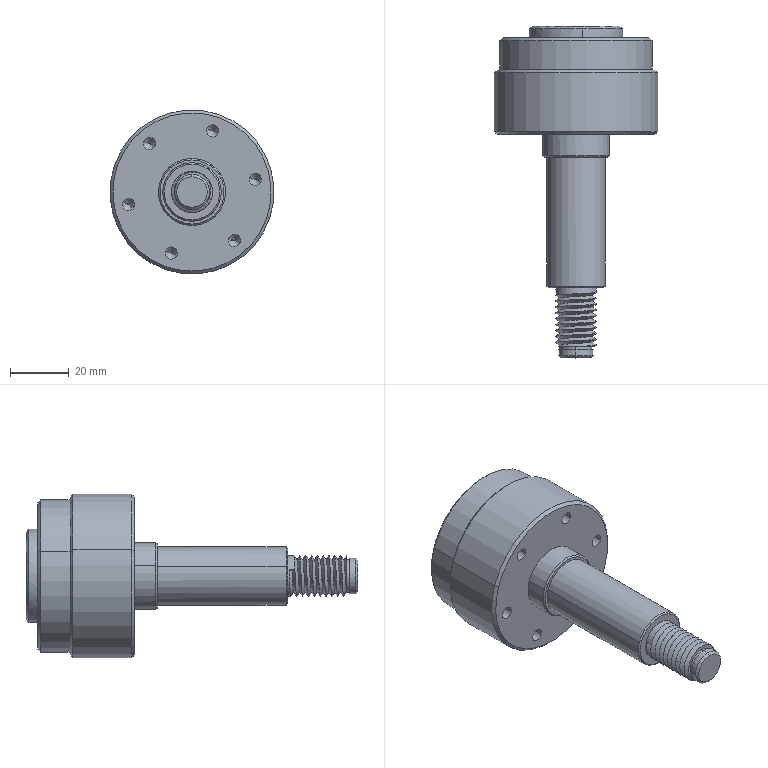Part | SolidWorks | features BaseBody 1 | 1 solid | 94 faces | box 56 x 113.25 x 56 mm | volume 96547 mm3 | cylinder 40 | cone 38 | plane 10 | spline 6 | commonest cylinder face diameters 4.2 x12 5 x12 11 x2 12 x2 14 x2 19.98 x2